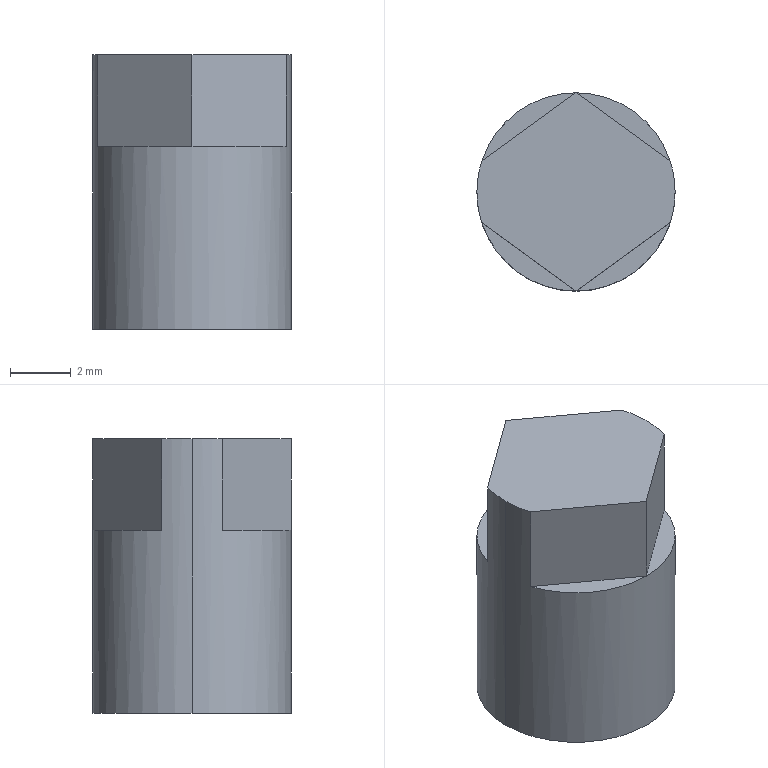Part | STEP file | Diamond pin | 1 solid | 16 faces | box 6.5 x 6.5 x 9 mm | volume 250.881 mm3 | plane 10 | cylinder 4 | cone 2 | commonest cylinder face diameters 2.9 x2 6.5 x2
STEP:
#1=CARTESIAN_POINT('',(1.45,0.,4.));
#2=VERTEX_POINT('',#1);
#3=CARTESIAN_POINT('',(-1.45,0.,4.));
#4=VERTEX_POINT('',#3);
#5=CARTESIAN_POINT('',(0.,0.,4.));
#6=DIRECTION('',(0.,0.,-1.));
#7=DIRECTION('',(-1.,0.,0.));
#8=AXIS2_PLACEMENT_3D('',#5,#6,#7);
#9=CIRCLE('',#8,1.45);
#10=EDGE_CURVE('',#2,#4,#9,.T.);
#11=ORIENTED_EDGE('',*,*,#10,.F.);
#12=CARTESIAN_POINT('',(1.45,0.,0.));
#13=VERTEX_POINT('',#12);
#14=CARTESIAN_POINT('',(1.45,0.,0.));
#15=DIRECTION('',(0.,0.,-1.));
#16=VECTOR('',#15,1000.);
#17=LINE('',#14,#16);
#18=EDGE_CURVE('',#2,#13,#17,.T.);
#19=ORIENTED_EDGE('',*,*,#18,.T.);
#20=CARTESIAN_POINT('',(-1.45,0.,0.));
#21=VERTEX_POINT('',#20);
#22=CARTESIAN_POINT('',(0.,0.,0.));
#23=DIRECTION('',(0.,0.,-1.));
#24=DIRECTION('',(-1.,0.,0.));
#25=AXIS2_PLACEMENT_3D('',#22,#23,#24);
#26=CIRCLE('',#25,1.45);
#27=EDGE_CURVE('',#13,#21,#26,.T.);
#28=ORIENTED_EDGE('',*,*,#27,.T.);
#29=CARTESIAN_POINT('',(-1.45,0.,0.));
#30=DIRECTION('',(0.,0.,-1.));
#31=VECTOR('',#30,1000.);
#32=LINE('',#29,#31);
#33=EDGE_CURVE('',#4,#21,#32,.T.);
#34=ORIENTED_EDGE('',*,*,#33,.F.);
#35=EDGE_LOOP('',(#11,#19,#28,#34));
#36=FACE_OUTER_BOUND('',#35,.T.);
#37=CARTESIAN_POINT('',(0.,0.,0.));
#38=DIRECTION('',(0.,0.,-1.));
#39=DIRECTION('',(-1.,0.,0.));
#40=AXIS2_PLACEMENT_3D('',#37,#38,#39);
#41=CYLINDRICAL_SURFACE('',#40,1.45);
#42=ADVANCED_FACE('',(#36),#41,.F.);
#43=CARTESIAN_POINT('',(0.,0.,4.871));
#44=VERTEX_POINT('',#43);
#45=CARTESIAN_POINT('',(-1.45,0.,4.));
#46=DIRECTION('',(-0.8572,0.,-0.515));
#47=VECTOR('',#46,1000.);
#48=LINE('',#45,#47);
#49=EDGE_CURVE('',#44,#4,#48,.T.);
#50=ORIENTED_EDGE('',*,*,#49,.F.);
#51=CARTESIAN_POINT('',(1.45,0.,4.));
#52=DIRECTION('',(0.8572,0.,-0.515));
#53=VECTOR('',#52,1000.);
#54=LINE('',#51,#53);
#55=EDGE_CURVE('',#44,#2,#54,.T.);
#56=ORIENTED_EDGE('',*,*,#55,.T.);
#57=ORIENTED_EDGE('',*,*,#10,.T.);
#58=EDGE_LOOP('',(#50,#56,#57));
#59=FACE_OUTER_BOUND('',#58,.T.);
#60=CARTESIAN_POINT('',(0.,0.,4.));
#61=DIRECTION('',(0.,0.,-1.));
#62=DIRECTION('',(-1.,0.,0.));
#63=AXIS2_PLACEMENT_3D('',#60,#61,#62);
#64=CONICAL_SURFACE('',#63,1.45,1.03);
#65=ADVANCED_FACE('',(#59),#64,.F.);
#66=CARTESIAN_POINT('',(3.25,0.,9.));
#67=VERTEX_POINT('',#66);
#68=CARTESIAN_POINT('',(3.092,1.,9.));
#69=VERTEX_POINT('',#68);
#70=CARTESIAN_POINT('',(0.,0.,9.));
#71=DIRECTION('',(0.,0.,1.));
#72=DIRECTION('',(1.,0.,0.));
#73=AXIS2_PLACEMENT_3D('',#70,#71,#72);
#74=CIRCLE('',#73,3.25);
#75=EDGE_CURVE('',#67,#69,#74,.T.);
#76=ORIENTED_EDGE('',*,*,#75,.F.);
#77=CARTESIAN_POINT('',(3.25,0.,0.));
#78=VERTEX_POINT('',#77);
#79=CARTESIAN_POINT('',(3.25,0.,9.));
#80=DIRECTION('',(0.,0.,-1.));
#81=VECTOR('',#80,1000.);
#82=LINE('',#79,#81);
#83=EDGE_CURVE('',#67,#78,#82,.T.);
#84=ORIENTED_EDGE('',*,*,#83,.T.);
#85=CARTESIAN_POINT('',(-3.25,0.,0.));
#86=VERTEX_POINT('',#85);
#87=CARTESIAN_POINT('',(0.,0.,0.));
#88=DIRECTION('',(0.,0.,1.));
#89=DIRECTION('',(1.,0.,0.));
#90=AXIS2_PLACEMENT_3D('',#87,#88,#89);
#91=CIRCLE('',#90,3.25);
#92=EDGE_CURVE('',#78,#86,#91,.T.);
#93=ORIENTED_EDGE('',*,*,#92,.T.);
#94=CARTESIAN_POINT('',(-3.25,0.,9.));
#95=VERTEX_POINT('',#94);
#96=CARTESIAN_POINT('',(-3.25,0.,9.));
#97=DIRECTION('',(0.,0.,-1.));
#98=VECTOR('',#97,1000.);
#99=LINE('',#96,#98);
#100=EDGE_CURVE('',#95,#86,#99,.T.);
#101=ORIENTED_EDGE('',*,*,#100,.F.);
#102=CARTESIAN_POINT('',(-3.092,1.,9.));
#103=VERTEX_POINT('',#102);
#104=CARTESIAN_POINT('',(0.,0.,9.));
#105=DIRECTION('',(0.,0.,1.));
#106=DIRECTION('',(1.,0.,0.));
#107=AXIS2_PLACEMENT_3D('',#104,#105,#106);
#108=CIRCLE('',#107,3.25);
#109=EDGE_CURVE('',#103,#95,#108,.T.);
#110=ORIENTED_EDGE('',*,*,#109,.F.);
#111=CARTESIAN_POINT('',(-3.092,1.,6.));
#112=VERTEX_POINT('',#111);
#113=CARTESIAN_POINT('',(-3.092,1.,6.));
#114=DIRECTION('',(0.,0.,1.));
#115=VECTOR('',#114,1000.);
#116=LINE('',#113,#115);
#117=EDGE_CURVE('',#112,#103,#116,.T.);
#118=ORIENTED_EDGE('',*,*,#117,.F.);
#119=CARTESIAN_POINT('',(0.,3.25,6.));
#120=VERTEX_POINT('',#119);
#121=CARTESIAN_POINT('',(0.,0.,6.));
#122=DIRECTION('',(0.,0.,1.));
#123=DIRECTION('',(1.,0.,0.));
#124=AXIS2_PLACEMENT_3D('',#121,#122,#123);
#125=CIRCLE('',#124,3.25);
#126=EDGE_CURVE('',#120,#112,#125,.T.);
#127=ORIENTED_EDGE('',*,*,#126,.F.);
#128=CARTESIAN_POINT('',(3.092,1.,6.));
#129=VERTEX_POINT('',#128);
#130=CARTESIAN_POINT('',(0.,0.,6.));
#131=DIRECTION('',(0.,0.,1.));
#132=DIRECTION('',(1.,0.,0.));
#133=AXIS2_PLACEMENT_3D('',#130,#131,#132);
#134=CIRCLE('',#133,3.25);
#135=EDGE_CURVE('',#129,#120,#134,.T.);
#136=ORIENTED_EDGE('',*,*,#135,.F.);
#137=CARTESIAN_POINT('',(3.092,1.,6.));
#138=DIRECTION('',(0.,0.,1.));
#139=VECTOR('',#138,1000.);
#140=LINE('',#137,#139);
#141=EDGE_CURVE('',#129,#69,#140,.T.);
#142=ORIENTED_EDGE('',*,*,#141,.T.);
#143=EDGE_LOOP('',(#76,#84,#93,#101,#110,#118,#127,#136,#142));
#144=FACE_OUTER_BOUND('',#143,.T.);
#145=CARTESIAN_POINT('',(0.,0.,9.));
#146=DIRECTION('',(0.,0.,-1.));
#147=DIRECTION('',(-1.,0.,0.));
#148=AXIS2_PLACEMENT_3D('',#145,#146,#147);
#149=CYLINDRICAL_SURFACE('',#148,3.25);
#150=ADVANCED_FACE('',(#144),#149,.T.);
#151=ORIENTED_EDGE('',*,*,#83,.F.);
#152=CARTESIAN_POINT('',(3.092,-1.,9.));
#153=VERTEX_POINT('',#152);
#154=CARTESIAN_POINT('',(0.,0.,9.));
#155=DIRECTION('',(0.,0.,1.));
#156=DIRECTION('',(1.,0.,0.));
#157=AXIS2_PLACEMENT_3D('',#154,#155,#156);
#158=CIRCLE('',#157,3.25);
#159=EDGE_CURVE('',#153,#67,#158,.T.);
#160=ORIENTED_EDGE('',*,*,#159,.F.);
#161=CARTESIAN_POINT('',(3.092,-1.,6.));
#162=VERTEX_POINT('',#161);
#163=CARTESIAN_POINT('',(3.092,-1.,6.));
#164=DIRECTION('',(0.,0.,1.));
#165=VECTOR('',#164,1000.);
#166=LINE('',#163,#165);
#167=EDGE_CURVE('',#162,#153,#166,.T.);
#168=ORIENTED_EDGE('',*,*,#167,.F.);
#169=CARTESIAN_POINT('',(0.,-3.25,6.));
#170=VERTEX_POINT('',#169);
#171=CARTESIAN_POINT('',(0.,0.,6.));
#172=DIRECTION('',(0.,0.,1.));
#173=DIRECTION('',(1.,0.,0.));
#174=AXIS2_PLACEMENT_3D('',#171,#172,#173);
#175=CIRCLE('',#174,3.25);
#176=EDGE_CURVE('',#170,#162,#175,.T.);
#177=ORIENTED_EDGE('',*,*,#176,.F.);
#178=CARTESIAN_POINT('',(-3.092,-1.,6.));
#179=VERTEX_POINT('',#178);
#180=CARTESIAN_POINT('',(0.,0.,6.));
#181=DIRECTION('',(0.,0.,1.));
#182=DIRECTION('',(1.,0.,0.));
#183=AXIS2_PLACEMENT_3D('',#180,#181,#182);
#184=CIRCLE('',#183,3.25);
#185=EDGE_CURVE('',#179,#170,#184,.T.);
#186=ORIENTED_EDGE('',*,*,#185,.F.);
#187=CARTESIAN_POINT('',(-3.092,-1.,9.));
#188=VERTEX_POINT('',#187);
#189=CARTESIAN_POINT('',(-3.092,-1.,6.));
#190=DIRECTION('',(0.,0.,1.));
#191=VECTOR('',#190,1000.);
#192=LINE('',#189,#191);
#193=EDGE_CURVE('',#179,#188,#192,.T.);
#194=ORIENTED_EDGE('',*,*,#193,.T.);
#195=CARTESIAN_POINT('',(0.,0.,9.));
#196=DIRECTION('',(0.,0.,1.));
#197=DIRECTION('',(1.,0.,0.));
#198=AXIS2_PLACEMENT_3D('',#195,#196,#197);
#199=CIRCLE('',#198,3.25);
#200=EDGE_CURVE('',#95,#188,#199,.T.);
#201=ORIENTED_EDGE('',*,*,#200,.F.);
#202=ORIENTED_EDGE('',*,*,#100,.T.);
#203=CARTESIAN_POINT('',(0.,0.,0.));
#204=DIRECTION('',(0.,0.,1.));
#205=DIRECTION('',(1.,0.,0.));
#206=AXIS2_PLACEMENT_3D('',#203,#204,#205);
#207=CIRCLE('',#206,3.25);
#208=EDGE_CURVE('',#86,#78,#207,.T.);
#209=ORIENTED_EDGE('',*,*,#208,.T.);
#210=EDGE_LOOP('',(#151,#160,#168,#177,#186,#194,#201,#202,#209));
#211=FACE_OUTER_BOUND('',#210,.T.);
#212=CARTESIAN_POINT('',(0.,0.,9.));
#213=DIRECTION('',(0.,0.,-1.));
#214=DIRECTION('',(-1.,0.,0.));
#215=AXIS2_PLACEMENT_3D('',#212,#213,#214);
#216=CYLINDRICAL_SURFACE('',#215,3.25);
#217=ADVANCED_FACE('',(#211),#216,.T.);
#218=CARTESIAN_POINT('',(0.,3.25,9.));
#219=VERTEX_POINT('',#218);
#220=CARTESIAN_POINT('',(-1.546,2.125,9.));
#221=DIRECTION('',(0.8086,0.5883,0.));
#222=VECTOR('',#221,1000.);
#223=LINE('',#220,#222);
#224=EDGE_CURVE('',#103,#219,#223,.T.);
#225=ORIENTED_EDGE('',*,*,#224,.F.);
#226=ORIENTED_EDGE('',*,*,#109,.T.);
#227=ORIENTED_EDGE('',*,*,#200,.T.);
#228=CARTESIAN_POINT('',(0.,-3.25,9.));
#229=VERTEX_POINT('',#228);
#230=CARTESIAN_POINT('',(-1.546,-2.125,9.));
#231=DIRECTION('',(0.8086,-0.5883,0.));
#232=VECTOR('',#231,1000.);
#233=LINE('',#230,#232);
#234=EDGE_CURVE('',#188,#229,#233,.T.);
#235=ORIENTED_EDGE('',*,*,#234,.T.);
#236=CARTESIAN_POINT('',(1.546,-2.125,9.));
#237=DIRECTION('',(0.8086,0.5883,0.));
#238=VECTOR('',#237,1000.);
#239=LINE('',#236,#238);
#240=EDGE_CURVE('',#229,#153,#239,.T.);
#241=ORIENTED_EDGE('',*,*,#240,.T.);
#242=ORIENTED_EDGE('',*,*,#159,.T.);
#243=ORIENTED_EDGE('',*,*,#75,.T.);
#244=CARTESIAN_POINT('',(1.546,2.125,9.));
#245=DIRECTION('',(0.8086,-0.5883,0.));
#246=VECTOR('',#245,1000.);
#247=LINE('',#244,#246);
#248=EDGE_CURVE('',#219,#69,#247,.T.);
#249=ORIENTED_EDGE('',*,*,#248,.F.);
#250=EDGE_LOOP('',(#225,#226,#227,#235,#241,#242,#243,#249));
#251=FACE_OUTER_BOUND('',#250,.T.);
#252=CARTESIAN_POINT('',(0.,0.,9.));
#253=DIRECTION('',(0.,0.,1.));
#254=DIRECTION('',(1.,0.,0.));
#255=AXIS2_PLACEMENT_3D('',#252,#253,#254);
#256=PLANE('',#255);
#257=ADVANCED_FACE('',(#251),#256,.T.);
#258=CARTESIAN_POINT('',(0.,0.,0.));
#259=DIRECTION('',(0.,0.,-1.));
#260=DIRECTION('',(-1.,0.,0.));
#261=AXIS2_PLACEMENT_3D('',#258,#259,#260);
#262=CIRCLE('',#261,1.45);
#263=EDGE_CURVE('',#21,#13,#262,.T.);
#264=ORIENTED_EDGE('',*,*,#263,.F.);
#265=ORIENTED_EDGE('',*,*,#27,.F.);
#266=EDGE_LOOP('',(#264,#265));
#267=FACE_BOUND('',#266,.T.);
#268=ORIENTED_EDGE('',*,*,#208,.F.);
#269=ORIENTED_EDGE('',*,*,#92,.F.);
#270=EDGE_LOOP('',(#268,#269));
#271=FACE_OUTER_BOUND('',#270,.T.);
#272=CARTESIAN_POINT('',(0.,0.,0.));
#273=DIRECTION('',(0.,0.,1.));
#274=DIRECTION('',(1.,0.,0.));
#275=AXIS2_PLACEMENT_3D('',#272,#273,#274);
#276=PLANE('',#275);
#277=ADVANCED_FACE('',(#267,#271),#276,.F.);
#278=ORIENTED_EDGE('',*,*,#240,.F.);
#279=CARTESIAN_POINT('',(0.,-3.25,6.));
#280=DIRECTION('',(0.,0.,1.));
#281=VECTOR('',#280,1000.);
#282=LINE('',#279,#281);
#283=EDGE_CURVE('',#170,#229,#282,.T.);
#284=ORIENTED_EDGE('',*,*,#283,.F.);
#285=CARTESIAN_POINT('',(1.546,-2.125,6.));
#286=DIRECTION('',(0.8086,0.5883,0.));
#287=VECTOR('',#286,1000.);
#288=LINE('',#285,#287);
#289=EDGE_CURVE('',#170,#162,#288,.T.);
#290=ORIENTED_EDGE('',*,*,#289,.T.);
#291=ORIENTED_EDGE('',*,*,#167,.T.);
#292=EDGE_LOOP('',(#278,#284,#290,#291));
#293=FACE_OUTER_BOUND('',#292,.T.);
#294=CARTESIAN_POINT('',(1.546,-2.125,6.));
#295=DIRECTION('',(0.5883,-0.8086,0.));
#296=DIRECTION('',(0.8086,0.5883,0.));
#297=AXIS2_PLACEMENT_3D('',#294,#295,#296);
#298=PLANE('',#297);
#299=ADVANCED_FACE('',(#293),#298,.T.);
#300=ORIENTED_EDGE('',*,*,#289,.F.);
#301=ORIENTED_EDGE('',*,*,#176,.T.);
#302=EDGE_LOOP('',(#300,#301));
#303=FACE_OUTER_BOUND('',#302,.T.);
#304=CARTESIAN_POINT('',(0.,0.,6.));
#305=DIRECTION('',(0.,0.,1.));
#306=DIRECTION('',(1.,0.,0.));
#307=AXIS2_PLACEMENT_3D('',#304,#305,#306);
#308=PLANE('',#307);
#309=ADVANCED_FACE('',(#303),#308,.T.);
#310=ORIENTED_EDGE('',*,*,#248,.T.);
#311=ORIENTED_EDGE('',*,*,#141,.F.);
#312=CARTESIAN_POINT('',(1.546,2.125,6.));
#313=DIRECTION('',(0.8086,-0.5883,0.));
#314=VECTOR('',#313,1000.);
#315=LINE('',#312,#314);
#316=EDGE_CURVE('',#120,#129,#315,.T.);
#317=ORIENTED_EDGE('',*,*,#316,.F.);
#318=CARTESIAN_POINT('',(0.,3.25,6.));
#319=DIRECTION('',(0.,0.,1.));
#320=VECTOR('',#319,1000.);
#321=LINE('',#318,#320);
#322=EDGE_CURVE('',#120,#219,#321,.T.);
#323=ORIENTED_EDGE('',*,*,#322,.T.);
#324=EDGE_LOOP('',(#310,#311,#317,#323));
#325=FACE_OUTER_BOUND('',#324,.T.);
#326=CARTESIAN_POINT('',(1.546,2.125,6.));
#327=DIRECTION('',(-0.5883,-0.8086,0.));
#328=DIRECTION('',(0.8086,-0.5883,0.));
#329=AXIS2_PLACEMENT_3D('',#326,#327,#328);
#330=PLANE('',#329);
#331=ADVANCED_FACE('',(#325),#330,.F.);
#332=ORIENTED_EDGE('',*,*,#135,.T.);
#333=ORIENTED_EDGE('',*,*,#316,.T.);
#334=EDGE_LOOP('',(#332,#333));
#335=FACE_OUTER_BOUND('',#334,.T.);
#336=CARTESIAN_POINT('',(0.,0.,6.));
#337=DIRECTION('',(0.,0.,1.));
#338=DIRECTION('',(1.,0.,0.));
#339=AXIS2_PLACEMENT_3D('',#336,#337,#338);
#340=PLANE('',#339);
#341=ADVANCED_FACE('',(#335),#340,.T.);
#342=ORIENTED_EDGE('',*,*,#224,.T.);
#343=ORIENTED_EDGE('',*,*,#322,.F.);
#344=CARTESIAN_POINT('',(-1.546,2.125,6.));
#345=DIRECTION('',(0.8086,0.5883,0.));
#346=VECTOR('',#345,1000.);
#347=LINE('',#344,#346);
#348=EDGE_CURVE('',#112,#120,#347,.T.);
#349=ORIENTED_EDGE('',*,*,#348,.F.);
#350=ORIENTED_EDGE('',*,*,#117,.T.);
#351=EDGE_LOOP('',(#342,#343,#349,#350));
#352=FACE_OUTER_BOUND('',#351,.T.);
#353=CARTESIAN_POINT('',(-1.546,2.125,6.));
#354=DIRECTION('',(0.5883,-0.8086,0.));
#355=DIRECTION('',(0.8086,0.5883,0.));
#356=AXIS2_PLACEMENT_3D('',#353,#354,#355);
#357=PLANE('',#356);
#358=ADVANCED_FACE('',(#352),#357,.F.);
#359=ORIENTED_EDGE('',*,*,#126,.T.);
#360=ORIENTED_EDGE('',*,*,#348,.T.);
#361=EDGE_LOOP('',(#359,#360));
#362=FACE_OUTER_BOUND('',#361,.T.);
#363=CARTESIAN_POINT('',(0.,0.,6.));
#364=DIRECTION('',(0.,0.,1.));
#365=DIRECTION('',(1.,0.,0.));
#366=AXIS2_PLACEMENT_3D('',#363,#364,#365);
#367=PLANE('',#366);
#368=ADVANCED_FACE('',(#362),#367,.T.);
#369=ORIENTED_EDGE('',*,*,#234,.F.);
#370=ORIENTED_EDGE('',*,*,#193,.F.);
#371=CARTESIAN_POINT('',(-1.546,-2.125,6.));
#372=DIRECTION('',(0.8086,-0.5883,0.));
#373=VECTOR('',#372,1000.);
#374=LINE('',#371,#373);
#375=EDGE_CURVE('',#179,#170,#374,.T.);
#376=ORIENTED_EDGE('',*,*,#375,.T.);
#377=ORIENTED_EDGE('',*,*,#283,.T.);
#378=EDGE_LOOP('',(#369,#370,#376,#377));
#379=FACE_OUTER_BOUND('',#378,.T.);
#380=CARTESIAN_POINT('',(-1.546,-2.125,6.));
#381=DIRECTION('',(-0.5883,-0.8086,0.));
#382=DIRECTION('',(0.8086,-0.5883,0.));
#383=AXIS2_PLACEMENT_3D('',#380,#381,#382);
#384=PLANE('',#383);
#385=ADVANCED_FACE('',(#379),#384,.T.);
#386=ORIENTED_EDGE('',*,*,#375,.F.);
#387=ORIENTED_EDGE('',*,*,#185,.T.);
#388=EDGE_LOOP('',(#386,#387));
#389=FACE_OUTER_BOUND('',#388,.T.);
#390=CARTESIAN_POINT('',(0.,0.,6.));
#391=DIRECTION('',(0.,0.,1.));
#392=DIRECTION('',(1.,0.,0.));
#393=AXIS2_PLACEMENT_3D('',#390,#391,#392);
#394=PLANE('',#393);
#395=ADVANCED_FACE('',(#389),#394,.T.);
#396=ORIENTED_EDGE('',*,*,#55,.F.);
#397=ORIENTED_EDGE('',*,*,#49,.T.);
#398=CARTESIAN_POINT('',(0.,0.,4.));
#399=DIRECTION('',(0.,0.,-1.));
#400=DIRECTION('',(-1.,0.,0.));
#401=AXIS2_PLACEMENT_3D('',#398,#399,#400);
#402=CIRCLE('',#401,1.45);
#403=EDGE_CURVE('',#4,#2,#402,.T.);
#404=ORIENTED_EDGE('',*,*,#403,.T.);
#405=EDGE_LOOP('',(#396,#397,#404));
#406=FACE_OUTER_BOUND('',#405,.T.);
#407=CARTESIAN_POINT('',(0.,0.,4.));
#408=DIRECTION('',(0.,0.,-1.));
#409=DIRECTION('',(-1.,0.,0.));
#410=AXIS2_PLACEMENT_3D('',#407,#408,#409);
#411=CONICAL_SURFACE('',#410,1.45,1.03);
#412=ADVANCED_FACE('',(#406),#411,.F.);
#413=ORIENTED_EDGE('',*,*,#18,.F.);
#414=ORIENTED_EDGE('',*,*,#403,.F.);
#415=ORIENTED_EDGE('',*,*,#33,.T.);
#416=ORIENTED_EDGE('',*,*,#263,.T.);
#417=EDGE_LOOP('',(#413,#414,#415,#416));
#418=FACE_OUTER_BOUND('',#417,.T.);
#419=CARTESIAN_POINT('',(0.,0.,0.));
#420=DIRECTION('',(0.,0.,-1.));
#421=DIRECTION('',(-1.,0.,0.));
#422=AXIS2_PLACEMENT_3D('',#419,#420,#421);
#423=CYLINDRICAL_SURFACE('',#422,1.45);
#424=ADVANCED_FACE('',(#418),#423,.F.);
#425=CLOSED_SHELL('',(#42,#65,#150,#217,#257,#277,#299,#309,#331,#341,#358,#368,#385,#395,#412,#424));
#426=MANIFOLD_SOLID_BREP('',#425);
#427=CARTESIAN_POINT('',(0.,0.,0.));
#428=DIRECTION('',(0.,0.,1.));
#429=DIRECTION('',(1.,0.,0.));
#430=AXIS2_PLACEMENT_3D('',#427,#428,#429);
#431=(LENGTH_UNIT()NAMED_UNIT(*)SI_UNIT(.MILLI.,.METRE.));
#432=UNCERTAINTY_MEASURE_WITH_UNIT(LENGTH_MEASURE(0.00001),#431,'','');
#433=(NAMED_UNIT(*)PLANE_ANGLE_UNIT()SI_UNIT($,.RADIAN.));
#434=(NAMED_UNIT(*)SI_UNIT($,.STERADIAN.)SOLID_ANGLE_UNIT());
#435=(GEOMETRIC_REPRESENTATION_CONTEXT(3)GLOBAL_UNCERTAINTY_ASSIGNED_CONTEXT((#432))GLOBAL_UNIT_ASSIGNED_CONTEXT((#431,#433,#434))REPRESENTATION_CONTEXT('',''));
#436=ADVANCED_BREP_SHAPE_REPRESENTATION('',(#426,#430),#435);